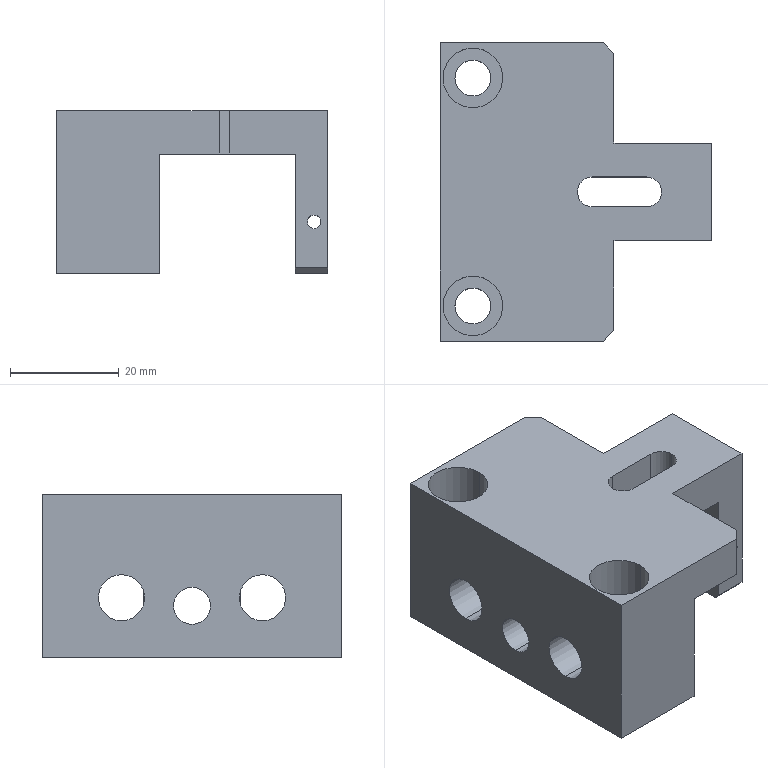Part | STEP file | 11-FG-B02511 | 1 solid | 60 faces | box 50 x 55 x 30 mm | volume 33514 mm3 | cylinder 35 | plane 25 | commonest cylinder face diameters 2.5 x10 5 x4 6.6 x4 8.5 x4 11 x4 5.5 x3